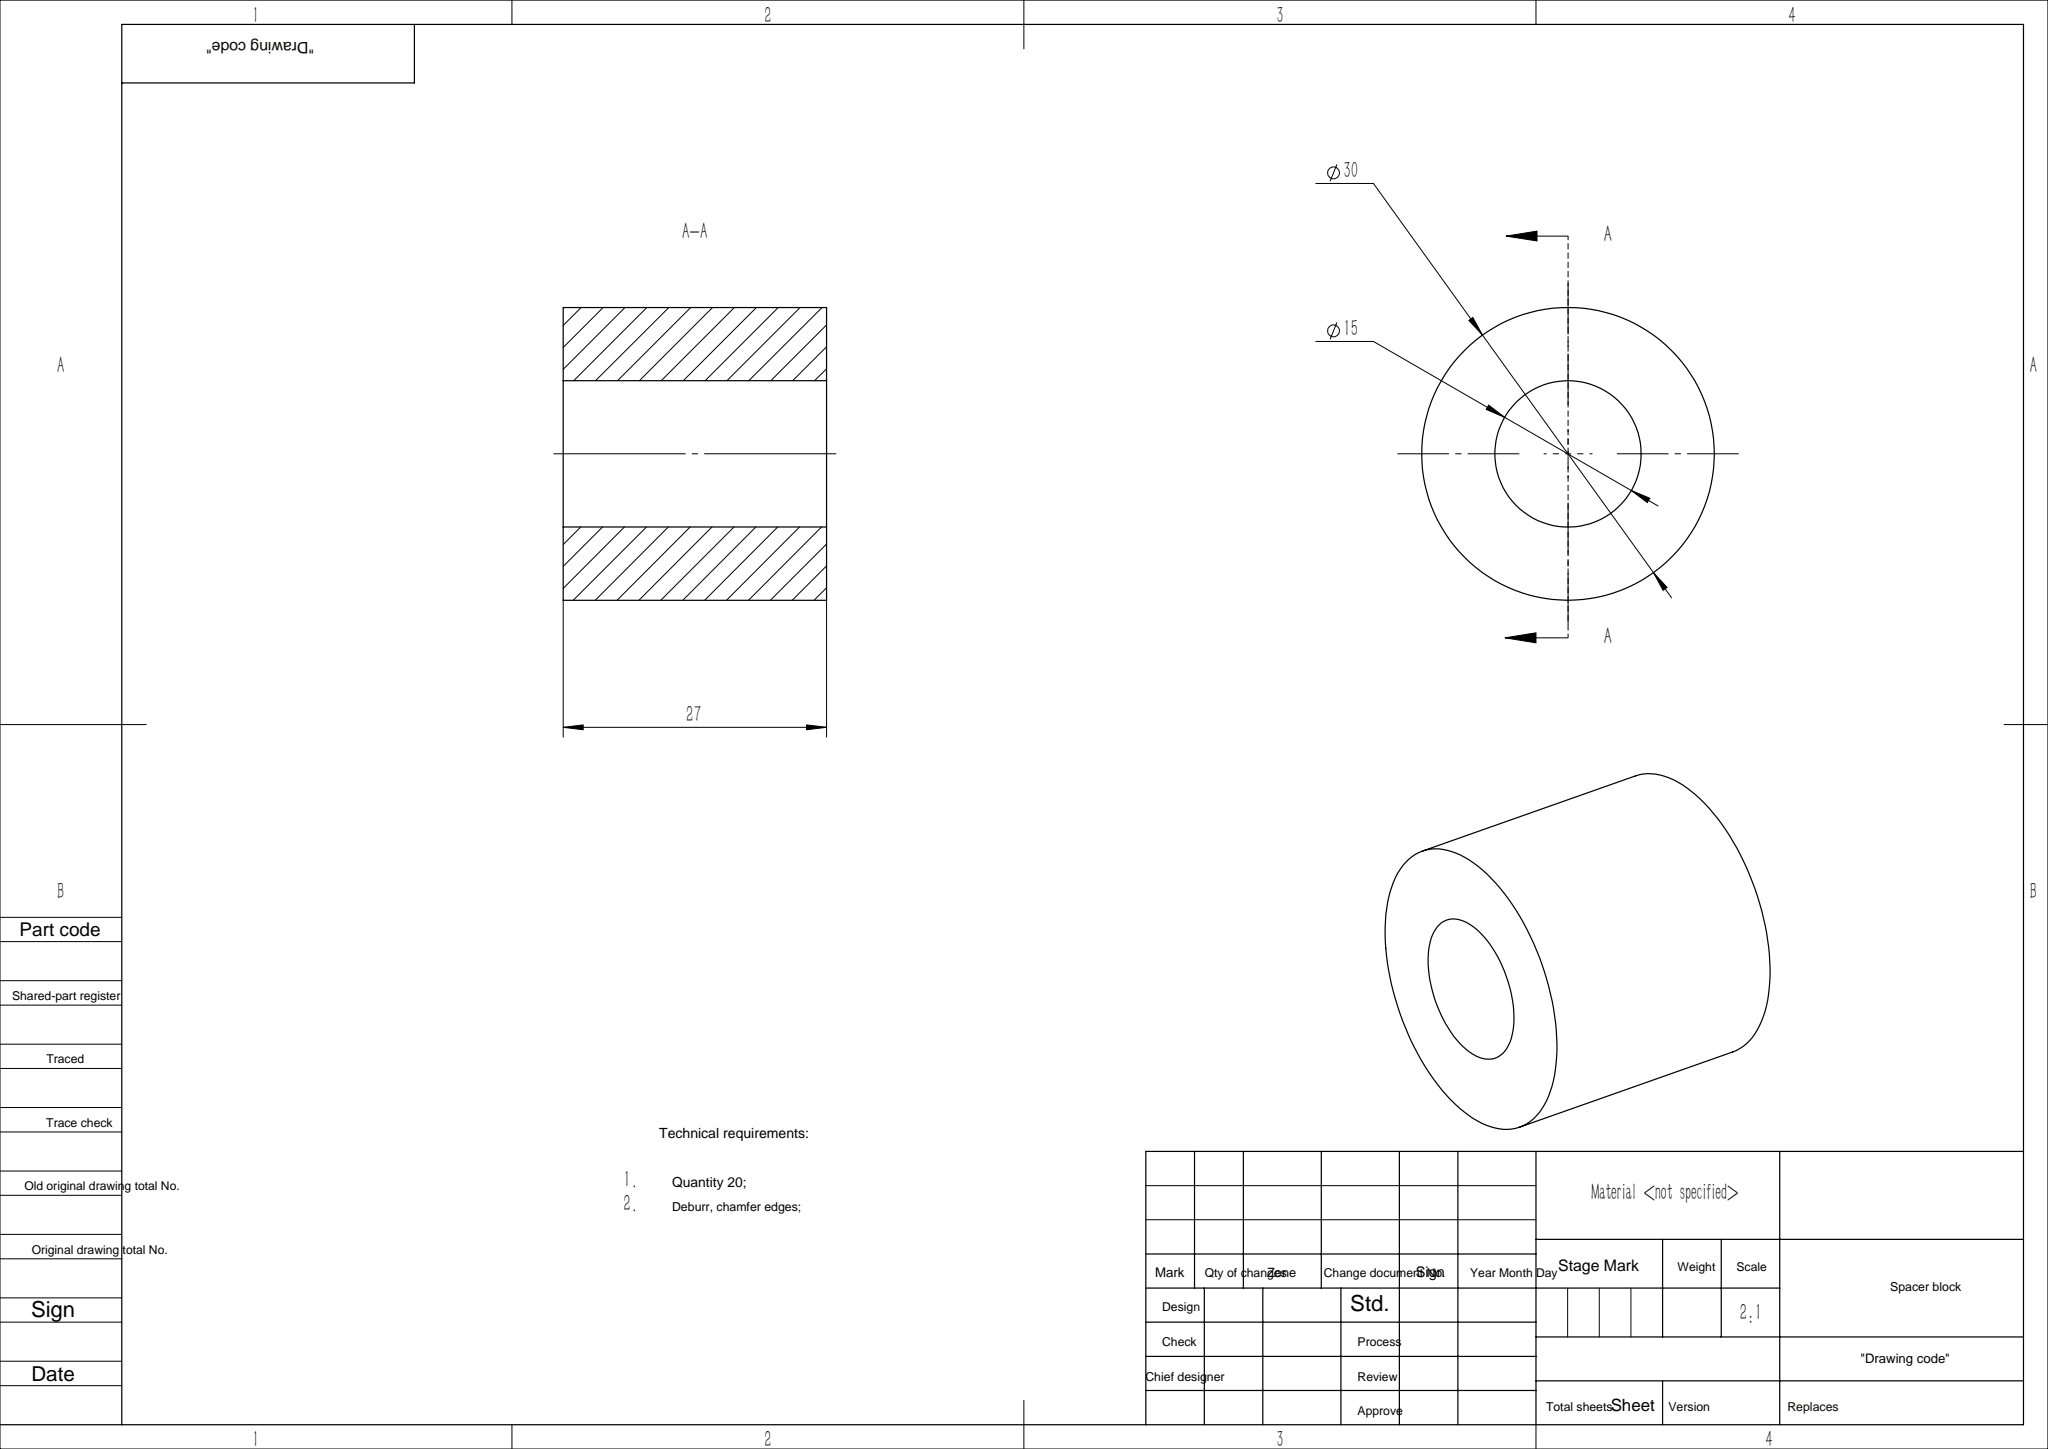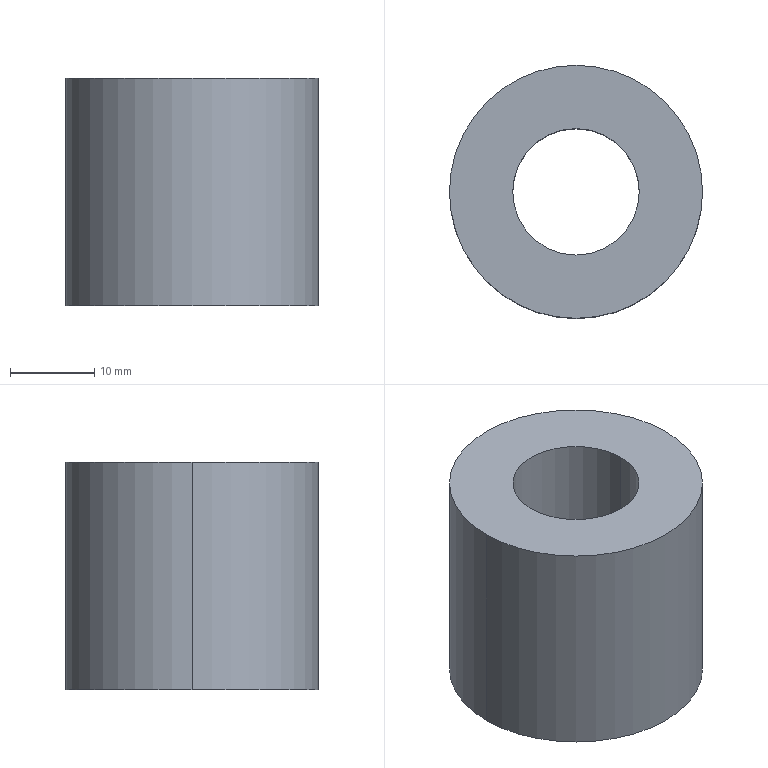Part | SolidWorks | features Extrusion 1 | 1 solid | 6 faces | box 30 x 30 x 27 mm | volume 14314 mm3 | cylinder 4 | plane 2 | commonest cylinder face diameters 15 x2 30 x2
STEP:
#1=CARTESIAN_POINT('',(653.439,1570.019,-498.));
#2=VERTEX_POINT('',#1);
#3=CARTESIAN_POINT('',(638.439,1570.019,-498.));
#4=VERTEX_POINT('',#3);
#5=CARTESIAN_POINT('',(645.939,1570.019,-498.));
#6=DIRECTION('',(0.,0.,-1.));
#7=DIRECTION('',(-1.,0.,0.));
#8=AXIS2_PLACEMENT_3D('',#5,#6,#7);
#9=CIRCLE('',#8,7.5);
#10=EDGE_CURVE('',#2,#4,#9,.T.);
#11=ORIENTED_EDGE('',*,*,#10,.T.);
#12=CARTESIAN_POINT('',(638.439,1570.019,-471.));
#13=VERTEX_POINT('',#12);
#14=CARTESIAN_POINT('',(638.439,1570.019,-540.426));
#15=DIRECTION('',(0.,0.,1.));
#16=VECTOR('',#15,1000.);
#17=LINE('',#14,#16);
#18=EDGE_CURVE('',#4,#13,#17,.T.);
#19=ORIENTED_EDGE('',*,*,#18,.T.);
#20=CARTESIAN_POINT('',(653.439,1570.019,-471.));
#21=VERTEX_POINT('',#20);
#22=CARTESIAN_POINT('',(645.939,1570.019,-471.));
#23=DIRECTION('',(0.,0.,-1.));
#24=DIRECTION('',(-1.,0.,0.));
#25=AXIS2_PLACEMENT_3D('',#22,#23,#24);
#26=CIRCLE('',#25,7.5);
#27=EDGE_CURVE('',#21,#13,#26,.T.);
#28=ORIENTED_EDGE('',*,*,#27,.F.);
#29=CARTESIAN_POINT('',(653.439,1570.019,-540.426));
#30=DIRECTION('',(0.,0.,1.));
#31=VECTOR('',#30,1000.);
#32=LINE('',#29,#31);
#33=EDGE_CURVE('',#2,#21,#32,.T.);
#34=ORIENTED_EDGE('',*,*,#33,.F.);
#35=EDGE_LOOP('',(#11,#19,#28,#34));
#36=FACE_OUTER_BOUND('',#35,.T.);
#37=CARTESIAN_POINT('',(645.939,1570.019,-540.426));
#38=DIRECTION('',(0.,0.,1.));
#39=DIRECTION('',(1.,0.,0.));
#40=AXIS2_PLACEMENT_3D('',#37,#38,#39);
#41=CYLINDRICAL_SURFACE('',#40,7.5);
#42=ADVANCED_FACE('',(#36),#41,.F.);
#43=CARTESIAN_POINT('',(660.939,1570.019,-498.));
#44=VERTEX_POINT('',#43);
#45=CARTESIAN_POINT('',(630.939,1570.019,-498.));
#46=VERTEX_POINT('',#45);
#47=CARTESIAN_POINT('',(645.939,1570.019,-498.));
#48=DIRECTION('',(0.,0.,1.));
#49=DIRECTION('',(1.,0.,0.));
#50=AXIS2_PLACEMENT_3D('',#47,#48,#49);
#51=CIRCLE('',#50,15.);
#52=EDGE_CURVE('',#44,#46,#51,.T.);
#53=ORIENTED_EDGE('',*,*,#52,.T.);
#54=CARTESIAN_POINT('',(630.939,1570.019,-471.));
#55=VERTEX_POINT('',#54);
#56=CARTESIAN_POINT('',(630.939,1570.019,-540.426));
#57=DIRECTION('',(0.,0.,1.));
#58=VECTOR('',#57,1000.);
#59=LINE('',#56,#58);
#60=EDGE_CURVE('',#46,#55,#59,.T.);
#61=ORIENTED_EDGE('',*,*,#60,.T.);
#62=CARTESIAN_POINT('',(660.939,1570.019,-471.));
#63=VERTEX_POINT('',#62);
#64=CARTESIAN_POINT('',(645.939,1570.019,-471.));
#65=DIRECTION('',(0.,0.,-1.));
#66=DIRECTION('',(-1.,0.,0.));
#67=AXIS2_PLACEMENT_3D('',#64,#65,#66);
#68=CIRCLE('',#67,15.);
#69=EDGE_CURVE('',#55,#63,#68,.T.);
#70=ORIENTED_EDGE('',*,*,#69,.T.);
#71=CARTESIAN_POINT('',(660.939,1570.019,-540.426));
#72=DIRECTION('',(0.,0.,1.));
#73=VECTOR('',#72,1000.);
#74=LINE('',#71,#73);
#75=EDGE_CURVE('',#44,#63,#74,.T.);
#76=ORIENTED_EDGE('',*,*,#75,.F.);
#77=EDGE_LOOP('',(#53,#61,#70,#76));
#78=FACE_OUTER_BOUND('',#77,.T.);
#79=CARTESIAN_POINT('',(645.939,1570.019,-540.426));
#80=DIRECTION('',(0.,0.,1.));
#81=DIRECTION('',(1.,0.,0.));
#82=AXIS2_PLACEMENT_3D('',#79,#80,#81);
#83=CYLINDRICAL_SURFACE('',#82,15.);
#84=ADVANCED_FACE('',(#78),#83,.T.);
#85=CARTESIAN_POINT('',(645.939,1570.019,-471.));
#86=DIRECTION('',(0.,0.,-1.));
#87=DIRECTION('',(-1.,0.,0.));
#88=AXIS2_PLACEMENT_3D('',#85,#86,#87);
#89=CIRCLE('',#88,15.);
#90=EDGE_CURVE('',#63,#55,#89,.T.);
#91=ORIENTED_EDGE('',*,*,#90,.F.);
#92=ORIENTED_EDGE('',*,*,#69,.F.);
#93=EDGE_LOOP('',(#91,#92));
#94=FACE_OUTER_BOUND('',#93,.T.);
#95=ORIENTED_EDGE('',*,*,#27,.T.);
#96=CARTESIAN_POINT('',(645.939,1570.019,-471.));
#97=DIRECTION('',(0.,0.,-1.));
#98=DIRECTION('',(-1.,0.,0.));
#99=AXIS2_PLACEMENT_3D('',#96,#97,#98);
#100=CIRCLE('',#99,7.5);
#101=EDGE_CURVE('',#13,#21,#100,.T.);
#102=ORIENTED_EDGE('',*,*,#101,.T.);
#103=EDGE_LOOP('',(#95,#102));
#104=FACE_BOUND('',#103,.T.);
#105=CARTESIAN_POINT('',(645.939,1570.019,-471.));
#106=DIRECTION('',(0.,0.,-1.));
#107=DIRECTION('',(-1.,0.,0.));
#108=AXIS2_PLACEMENT_3D('',#105,#106,#107);
#109=PLANE('',#108);
#110=ADVANCED_FACE('',(#94,#104),#109,.F.);
#111=ORIENTED_EDGE('',*,*,#60,.F.);
#112=CARTESIAN_POINT('',(645.939,1570.019,-498.));
#113=DIRECTION('',(0.,0.,1.));
#114=DIRECTION('',(1.,0.,0.));
#115=AXIS2_PLACEMENT_3D('',#112,#113,#114);
#116=CIRCLE('',#115,15.);
#117=EDGE_CURVE('',#46,#44,#116,.T.);
#118=ORIENTED_EDGE('',*,*,#117,.T.);
#119=ORIENTED_EDGE('',*,*,#75,.T.);
#120=ORIENTED_EDGE('',*,*,#90,.T.);
#121=EDGE_LOOP('',(#111,#118,#119,#120));
#122=FACE_OUTER_BOUND('',#121,.T.);
#123=CARTESIAN_POINT('',(645.939,1570.019,-540.426));
#124=DIRECTION('',(0.,0.,1.));
#125=DIRECTION('',(1.,0.,0.));
#126=AXIS2_PLACEMENT_3D('',#123,#124,#125);
#127=CYLINDRICAL_SURFACE('',#126,15.);
#128=ADVANCED_FACE('',(#122),#127,.T.);
#129=ORIENTED_EDGE('',*,*,#18,.F.);
#130=CARTESIAN_POINT('',(645.939,1570.019,-498.));
#131=DIRECTION('',(0.,0.,-1.));
#132=DIRECTION('',(-1.,0.,0.));
#133=AXIS2_PLACEMENT_3D('',#130,#131,#132);
#134=CIRCLE('',#133,7.5);
#135=EDGE_CURVE('',#4,#2,#134,.T.);
#136=ORIENTED_EDGE('',*,*,#135,.T.);
#137=ORIENTED_EDGE('',*,*,#33,.T.);
#138=ORIENTED_EDGE('',*,*,#101,.F.);
#139=EDGE_LOOP('',(#129,#136,#137,#138));
#140=FACE_OUTER_BOUND('',#139,.T.);
#141=CARTESIAN_POINT('',(645.939,1570.019,-540.426));
#142=DIRECTION('',(0.,0.,1.));
#143=DIRECTION('',(1.,0.,0.));
#144=AXIS2_PLACEMENT_3D('',#141,#142,#143);
#145=CYLINDRICAL_SURFACE('',#144,7.5);
#146=ADVANCED_FACE('',(#140),#145,.F.);
#147=ORIENTED_EDGE('',*,*,#10,.F.);
#148=ORIENTED_EDGE('',*,*,#135,.F.);
#149=EDGE_LOOP('',(#147,#148));
#150=FACE_BOUND('',#149,.T.);
#151=ORIENTED_EDGE('',*,*,#52,.F.);
#152=ORIENTED_EDGE('',*,*,#117,.F.);
#153=EDGE_LOOP('',(#151,#152));
#154=FACE_OUTER_BOUND('',#153,.T.);
#155=CARTESIAN_POINT('',(0.,0.,-498.));
#156=DIRECTION('',(0.,0.,1.));
#157=DIRECTION('',(1.,0.,0.));
#158=AXIS2_PLACEMENT_3D('',#155,#156,#157);
#159=PLANE('',#158);
#160=ADVANCED_FACE('',(#150,#154),#159,.F.);
#161=CLOSED_SHELL('',(#42,#84,#110,#128,#146,#160));
#162=MANIFOLD_SOLID_BREP('',#161);
#163=CARTESIAN_POINT('',(0.,0.,0.));
#164=DIRECTION('',(0.,0.,1.));
#165=DIRECTION('',(1.,0.,0.));
#166=AXIS2_PLACEMENT_3D('',#163,#164,#165);
#167=(LENGTH_UNIT()NAMED_UNIT(*)SI_UNIT(.MILLI.,.METRE.));
#168=UNCERTAINTY_MEASURE_WITH_UNIT(LENGTH_MEASURE(0.00001),#167,'','');
#169=(NAMED_UNIT(*)PLANE_ANGLE_UNIT()SI_UNIT($,.RADIAN.));
#170=(NAMED_UNIT(*)SI_UNIT($,.STERADIAN.)SOLID_ANGLE_UNIT());
#171=(GEOMETRIC_REPRESENTATION_CONTEXT(3)GLOBAL_UNCERTAINTY_ASSIGNED_CONTEXT((#168))GLOBAL_UNIT_ASSIGNED_CONTEXT((#167,#169,#170))REPRESENTATION_CONTEXT('',''));
#172=ADVANCED_BREP_SHAPE_REPRESENTATION('',(#162,#166),#171);